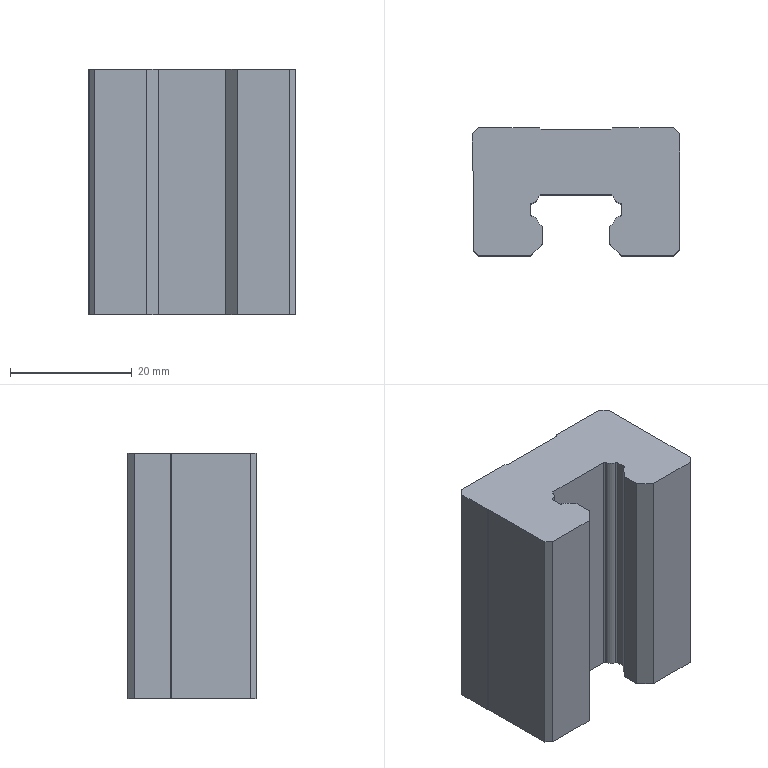Part | SolidWorks | features BaseBody 1 | 1 solid | 76 faces | box 34 x 21 x 40.2 mm | volume 22959 mm3 | plane 32 | cylinder 28 | cone 16 | commonest cylinder face diameters 0.6 x8 3.3 x8 4 x8 2.6 x4